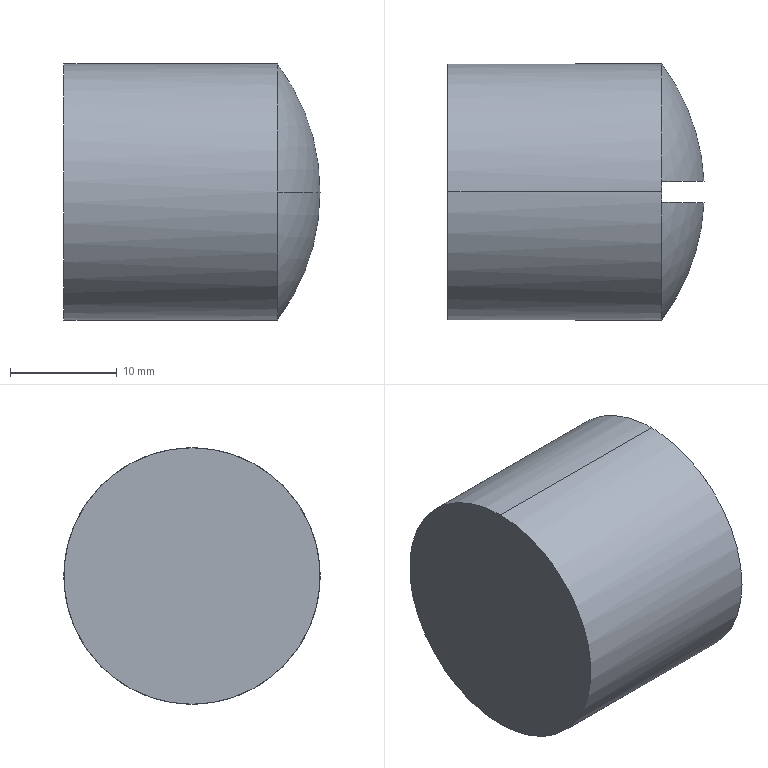Part | SolidWorks | features ICE 1, Revolution 1 | 1 solid | 10 faces | box 23.975 x 24 x 24 mm | volume 9856 mm3 | sphere 4 | plane 4 | cylinder 2 | commonest cylinder face diameters 24 x2
STEP:
#1=CARTESIAN_POINT('',(20.,-1.,-11.958));
#2=VERTEX_POINT('',#1);
#3=CARTESIAN_POINT('',(23.975,-1.,0.));
#4=VERTEX_POINT('',#3);
#5=CARTESIAN_POINT('',(4.,-1.,0.));
#6=DIRECTION('',(0.,-1.,0.));
#7=DIRECTION('',(0.,0.,-1.));
#8=AXIS2_PLACEMENT_3D('',#5,#6,#7);
#9=CIRCLE('',#8,19.975);
#10=EDGE_CURVE('',#2,#4,#9,.T.);
#11=ORIENTED_EDGE('',*,*,#10,.T.);
#12=CARTESIAN_POINT('',(20.,-12.,0.));
#13=VERTEX_POINT('',#12);
#14=CARTESIAN_POINT('',(4.,0.,0.));
#15=DIRECTION('',(0.,0.,-1.));
#16=DIRECTION('',(-1.,0.,0.));
#17=AXIS2_PLACEMENT_3D('',#14,#15,#16);
#18=CIRCLE('',#17,20.);
#19=EDGE_CURVE('',#4,#13,#18,.T.);
#20=ORIENTED_EDGE('',*,*,#19,.T.);
#21=CARTESIAN_POINT('',(20.,0.,0.));
#22=DIRECTION('',(-1.,0.,0.));
#23=DIRECTION('',(0.,0.,1.));
#24=AXIS2_PLACEMENT_3D('',#21,#22,#23);
#25=CIRCLE('',#24,12.);
#26=EDGE_CURVE('',#2,#13,#25,.T.);
#27=ORIENTED_EDGE('',*,*,#26,.F.);
#28=EDGE_LOOP('',(#11,#20,#27));
#29=FACE_OUTER_BOUND('',#28,.T.);
#30=CARTESIAN_POINT('',(4.,0.,0.));
#31=DIRECTION('',(0.,0.,1.));
#32=DIRECTION('',(0.,-1.,0.));
#33=AXIS2_PLACEMENT_3D('',#30,#31,#32);
#34=SPHERICAL_SURFACE('',#33,20.);
#35=ADVANCED_FACE('',(#29),#34,.T.);
#36=CARTESIAN_POINT('',(20.,1.,-11.958));
#37=VERTEX_POINT('',#36);
#38=CARTESIAN_POINT('',(20.,0.,-12.));
#39=VERTEX_POINT('',#38);
#40=CARTESIAN_POINT('',(20.,0.,0.));
#41=DIRECTION('',(-1.,0.,0.));
#42=DIRECTION('',(0.,0.,1.));
#43=AXIS2_PLACEMENT_3D('',#40,#41,#42);
#44=CIRCLE('',#43,12.);
#45=EDGE_CURVE('',#37,#39,#44,.T.);
#46=ORIENTED_EDGE('',*,*,#45,.T.);
#47=CARTESIAN_POINT('',(0.,0.,-12.));
#48=VERTEX_POINT('',#47);
#49=CARTESIAN_POINT('',(0.,0.,-12.));
#50=DIRECTION('',(-1.,0.,0.));
#51=VECTOR('',#50,1000.);
#52=LINE('',#49,#51);
#53=EDGE_CURVE('',#39,#48,#52,.T.);
#54=ORIENTED_EDGE('',*,*,#53,.T.);
#55=CARTESIAN_POINT('',(0.,0.,12.));
#56=VERTEX_POINT('',#55);
#57=CARTESIAN_POINT('',(0.,0.,0.));
#58=DIRECTION('',(-1.,0.,0.));
#59=DIRECTION('',(0.,0.,1.));
#60=AXIS2_PLACEMENT_3D('',#57,#58,#59);
#61=CIRCLE('',#60,12.);
#62=EDGE_CURVE('',#56,#48,#61,.T.);
#63=ORIENTED_EDGE('',*,*,#62,.F.);
#64=CARTESIAN_POINT('',(20.,0.,12.));
#65=VERTEX_POINT('',#64);
#66=CARTESIAN_POINT('',(0.,0.,12.));
#67=DIRECTION('',(-1.,0.,0.));
#68=VECTOR('',#67,1000.);
#69=LINE('',#66,#68);
#70=EDGE_CURVE('',#65,#56,#69,.T.);
#71=ORIENTED_EDGE('',*,*,#70,.F.);
#72=CARTESIAN_POINT('',(20.,1.,11.958));
#73=VERTEX_POINT('',#72);
#74=CARTESIAN_POINT('',(20.,0.,0.));
#75=DIRECTION('',(-1.,0.,0.));
#76=DIRECTION('',(0.,0.,1.));
#77=AXIS2_PLACEMENT_3D('',#74,#75,#76);
#78=CIRCLE('',#77,12.);
#79=EDGE_CURVE('',#65,#73,#78,.T.);
#80=ORIENTED_EDGE('',*,*,#79,.T.);
#81=CARTESIAN_POINT('',(20.,12.,0.));
#82=VERTEX_POINT('',#81);
#83=CARTESIAN_POINT('',(20.,0.,0.));
#84=DIRECTION('',(-1.,0.,0.));
#85=DIRECTION('',(0.,0.,1.));
#86=AXIS2_PLACEMENT_3D('',#83,#84,#85);
#87=CIRCLE('',#86,12.);
#88=EDGE_CURVE('',#73,#82,#87,.T.);
#89=ORIENTED_EDGE('',*,*,#88,.T.);
#90=CARTESIAN_POINT('',(20.,0.,0.));
#91=DIRECTION('',(-1.,0.,0.));
#92=DIRECTION('',(0.,0.,1.));
#93=AXIS2_PLACEMENT_3D('',#90,#91,#92);
#94=CIRCLE('',#93,12.);
#95=EDGE_CURVE('',#82,#37,#94,.T.);
#96=ORIENTED_EDGE('',*,*,#95,.T.);
#97=EDGE_LOOP('',(#46,#54,#63,#71,#80,#89,#96));
#98=FACE_OUTER_BOUND('',#97,.T.);
#99=CARTESIAN_POINT('',(0.,0.,0.));
#100=DIRECTION('',(-1.,0.,0.));
#101=DIRECTION('',(0.,0.,1.));
#102=AXIS2_PLACEMENT_3D('',#99,#100,#101);
#103=CYLINDRICAL_SURFACE('',#102,12.);
#104=ADVANCED_FACE('',(#98),#103,.T.);
#105=CARTESIAN_POINT('',(23.975,1.,0.));
#106=VERTEX_POINT('',#105);
#107=CARTESIAN_POINT('',(4.,1.,0.));
#108=DIRECTION('',(0.,1.,0.));
#109=DIRECTION('',(0.,0.,1.));
#110=AXIS2_PLACEMENT_3D('',#107,#108,#109);
#111=CIRCLE('',#110,19.975);
#112=EDGE_CURVE('',#73,#106,#111,.T.);
#113=ORIENTED_EDGE('',*,*,#112,.T.);
#114=CARTESIAN_POINT('',(4.,0.,0.));
#115=DIRECTION('',(0.,0.,1.));
#116=DIRECTION('',(0.,-1.,0.));
#117=AXIS2_PLACEMENT_3D('',#114,#115,#116);
#118=CIRCLE('',#117,20.);
#119=EDGE_CURVE('',#106,#82,#118,.T.);
#120=ORIENTED_EDGE('',*,*,#119,.T.);
#121=ORIENTED_EDGE('',*,*,#88,.F.);
#122=EDGE_LOOP('',(#113,#120,#121));
#123=FACE_OUTER_BOUND('',#122,.T.);
#124=CARTESIAN_POINT('',(4.,0.,0.));
#125=DIRECTION('',(0.,0.,1.));
#126=DIRECTION('',(0.,-1.,0.));
#127=AXIS2_PLACEMENT_3D('',#124,#125,#126);
#128=SPHERICAL_SURFACE('',#127,20.);
#129=ADVANCED_FACE('',(#123),#128,.T.);
#130=ORIENTED_EDGE('',*,*,#119,.F.);
#131=CARTESIAN_POINT('',(4.,1.,0.));
#132=DIRECTION('',(0.,1.,0.));
#133=DIRECTION('',(0.,0.,1.));
#134=AXIS2_PLACEMENT_3D('',#131,#132,#133);
#135=CIRCLE('',#134,19.975);
#136=EDGE_CURVE('',#106,#37,#135,.T.);
#137=ORIENTED_EDGE('',*,*,#136,.T.);
#138=ORIENTED_EDGE('',*,*,#95,.F.);
#139=EDGE_LOOP('',(#130,#137,#138));
#140=FACE_OUTER_BOUND('',#139,.T.);
#141=CARTESIAN_POINT('',(4.,0.,0.));
#142=DIRECTION('',(0.,0.,1.));
#143=DIRECTION('',(0.,-1.,0.));
#144=AXIS2_PLACEMENT_3D('',#141,#142,#143);
#145=SPHERICAL_SURFACE('',#144,20.);
#146=ADVANCED_FACE('',(#140),#145,.T.);
#147=ORIENTED_EDGE('',*,*,#62,.T.);
#148=CARTESIAN_POINT('',(0.,0.,0.));
#149=DIRECTION('',(-1.,0.,0.));
#150=DIRECTION('',(0.,0.,1.));
#151=AXIS2_PLACEMENT_3D('',#148,#149,#150);
#152=CIRCLE('',#151,12.);
#153=EDGE_CURVE('',#48,#56,#152,.T.);
#154=ORIENTED_EDGE('',*,*,#153,.T.);
#155=EDGE_LOOP('',(#147,#154));
#156=FACE_OUTER_BOUND('',#155,.T.);
#157=CARTESIAN_POINT('',(0.,0.,0.));
#158=DIRECTION('',(1.,0.,0.));
#159=DIRECTION('',(0.,0.,-1.));
#160=AXIS2_PLACEMENT_3D('',#157,#158,#159);
#161=PLANE('',#160);
#162=ADVANCED_FACE('',(#156),#161,.F.);
#163=ORIENTED_EDGE('',*,*,#53,.F.);
#164=CARTESIAN_POINT('',(20.,0.,0.));
#165=DIRECTION('',(-1.,0.,0.));
#166=DIRECTION('',(0.,0.,1.));
#167=AXIS2_PLACEMENT_3D('',#164,#165,#166);
#168=CIRCLE('',#167,12.);
#169=EDGE_CURVE('',#39,#2,#168,.T.);
#170=ORIENTED_EDGE('',*,*,#169,.T.);
#171=ORIENTED_EDGE('',*,*,#26,.T.);
#172=CARTESIAN_POINT('',(20.,-1.,11.958));
#173=VERTEX_POINT('',#172);
#174=CARTESIAN_POINT('',(20.,0.,0.));
#175=DIRECTION('',(-1.,0.,0.));
#176=DIRECTION('',(0.,0.,1.));
#177=AXIS2_PLACEMENT_3D('',#174,#175,#176);
#178=CIRCLE('',#177,12.);
#179=EDGE_CURVE('',#13,#173,#178,.T.);
#180=ORIENTED_EDGE('',*,*,#179,.T.);
#181=CARTESIAN_POINT('',(20.,0.,0.));
#182=DIRECTION('',(-1.,0.,0.));
#183=DIRECTION('',(0.,0.,1.));
#184=AXIS2_PLACEMENT_3D('',#181,#182,#183);
#185=CIRCLE('',#184,12.);
#186=EDGE_CURVE('',#173,#65,#185,.T.);
#187=ORIENTED_EDGE('',*,*,#186,.T.);
#188=ORIENTED_EDGE('',*,*,#70,.T.);
#189=ORIENTED_EDGE('',*,*,#153,.F.);
#190=EDGE_LOOP('',(#163,#170,#171,#180,#187,#188,#189));
#191=FACE_OUTER_BOUND('',#190,.T.);
#192=CARTESIAN_POINT('',(0.,0.,0.));
#193=DIRECTION('',(-1.,0.,0.));
#194=DIRECTION('',(0.,0.,1.));
#195=AXIS2_PLACEMENT_3D('',#192,#193,#194);
#196=CYLINDRICAL_SURFACE('',#195,12.);
#197=ADVANCED_FACE('',(#191),#196,.T.);
#198=ORIENTED_EDGE('',*,*,#19,.F.);
#199=CARTESIAN_POINT('',(4.,-1.,0.));
#200=DIRECTION('',(0.,-1.,0.));
#201=DIRECTION('',(0.,0.,-1.));
#202=AXIS2_PLACEMENT_3D('',#199,#200,#201);
#203=CIRCLE('',#202,19.975);
#204=EDGE_CURVE('',#4,#173,#203,.T.);
#205=ORIENTED_EDGE('',*,*,#204,.T.);
#206=ORIENTED_EDGE('',*,*,#179,.F.);
#207=EDGE_LOOP('',(#198,#205,#206));
#208=FACE_OUTER_BOUND('',#207,.T.);
#209=CARTESIAN_POINT('',(4.,0.,0.));
#210=DIRECTION('',(0.,0.,1.));
#211=DIRECTION('',(0.,-1.,0.));
#212=AXIS2_PLACEMENT_3D('',#209,#210,#211);
#213=SPHERICAL_SURFACE('',#212,20.);
#214=ADVANCED_FACE('',(#208),#213,.T.);
#215=CARTESIAN_POINT('',(20.,1.,-12.));
#216=DIRECTION('',(0.,0.,1.));
#217=VECTOR('',#216,1000.);
#218=LINE('',#215,#217);
#219=EDGE_CURVE('',#37,#73,#218,.T.);
#220=ORIENTED_EDGE('',*,*,#219,.T.);
#221=ORIENTED_EDGE('',*,*,#79,.F.);
#222=ORIENTED_EDGE('',*,*,#186,.F.);
#223=CARTESIAN_POINT('',(20.,-1.,-12.));
#224=DIRECTION('',(0.,0.,1.));
#225=VECTOR('',#224,1000.);
#226=LINE('',#223,#225);
#227=EDGE_CURVE('',#2,#173,#226,.T.);
#228=ORIENTED_EDGE('',*,*,#227,.F.);
#229=ORIENTED_EDGE('',*,*,#169,.F.);
#230=ORIENTED_EDGE('',*,*,#45,.F.);
#231=EDGE_LOOP('',(#220,#221,#222,#228,#229,#230));
#232=FACE_OUTER_BOUND('',#231,.T.);
#233=CARTESIAN_POINT('',(20.,-1.,-12.));
#234=DIRECTION('',(-1.,0.,0.));
#235=DIRECTION('',(0.,0.,1.));
#236=AXIS2_PLACEMENT_3D('',#233,#234,#235);
#237=PLANE('',#236);
#238=ADVANCED_FACE('',(#232),#237,.F.);
#239=ORIENTED_EDGE('',*,*,#219,.F.);
#240=ORIENTED_EDGE('',*,*,#136,.F.);
#241=ORIENTED_EDGE('',*,*,#112,.F.);
#242=EDGE_LOOP('',(#239,#240,#241));
#243=FACE_OUTER_BOUND('',#242,.T.);
#244=CARTESIAN_POINT('',(28.,1.,-12.));
#245=DIRECTION('',(0.,1.,0.));
#246=DIRECTION('',(0.,0.,1.));
#247=AXIS2_PLACEMENT_3D('',#244,#245,#246);
#248=PLANE('',#247);
#249=ADVANCED_FACE('',(#243),#248,.F.);
#250=ORIENTED_EDGE('',*,*,#227,.T.);
#251=ORIENTED_EDGE('',*,*,#204,.F.);
#252=ORIENTED_EDGE('',*,*,#10,.F.);
#253=EDGE_LOOP('',(#250,#251,#252));
#254=FACE_OUTER_BOUND('',#253,.T.);
#255=CARTESIAN_POINT('',(28.,-1.,-12.));
#256=DIRECTION('',(0.,-1.,0.));
#257=DIRECTION('',(0.,0.,-1.));
#258=AXIS2_PLACEMENT_3D('',#255,#256,#257);
#259=PLANE('',#258);
#260=ADVANCED_FACE('',(#254),#259,.F.);
#261=CLOSED_SHELL('',(#35,#104,#129,#146,#162,#197,#214,#238,#249,#260));
#262=MANIFOLD_SOLID_BREP('',#261);
#263=CARTESIAN_POINT('',(0.,0.,0.));
#264=DIRECTION('',(0.,0.,1.));
#265=DIRECTION('',(1.,0.,0.));
#266=AXIS2_PLACEMENT_3D('',#263,#264,#265);
#267=(LENGTH_UNIT()NAMED_UNIT(*)SI_UNIT(.MILLI.,.METRE.));
#268=UNCERTAINTY_MEASURE_WITH_UNIT(LENGTH_MEASURE(0.00001),#267,'','');
#269=(NAMED_UNIT(*)PLANE_ANGLE_UNIT()SI_UNIT($,.RADIAN.));
#270=(NAMED_UNIT(*)SI_UNIT($,.STERADIAN.)SOLID_ANGLE_UNIT());
#271=(GEOMETRIC_REPRESENTATION_CONTEXT(3)GLOBAL_UNCERTAINTY_ASSIGNED_CONTEXT((#268))GLOBAL_UNIT_ASSIGNED_CONTEXT((#267,#269,#270))REPRESENTATION_CONTEXT('',''));
#272=ADVANCED_BREP_SHAPE_REPRESENTATION('',(#262,#266),#271);